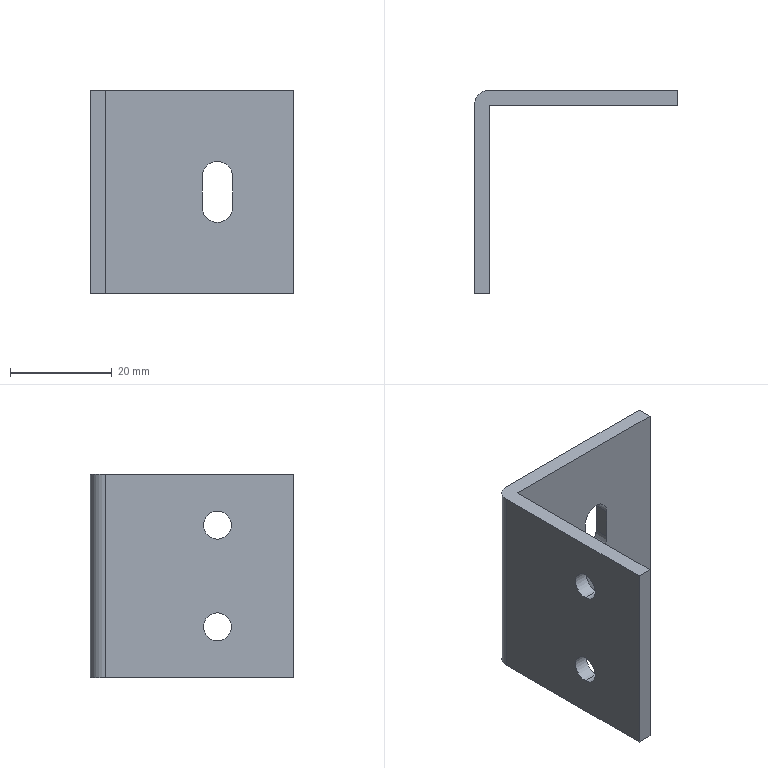Part | STEP file | 0245_212_Blacket | 1 solid | 18 faces | box 40 x 40 x 40 mm | volume 8827 mm3 | plane 10 | cylinder 8 | commonest cylinder face diameters 5.5 x4 6 x4
STEP:
#1=CARTESIAN_POINT('',(0.,0.,0.));
#2=DIRECTION('',(0.,0.,1.));
#3=DIRECTION('',(1.,0.,0.));
#4=AXIS2_PLACEMENT_3D('',#1,#2,#3);
#5=CARTESIAN_POINT('',(3.,15.,12.75));
#6=VERTEX_POINT('',#5);
#7=CARTESIAN_POINT('',(0.,15.,12.75));
#8=VERTEX_POINT('',#7);
#9=CARTESIAN_POINT('',(0.,15.,12.75));
#10=DIRECTION('',(-1.,0.,0.));
#11=VECTOR('',#10,1.);
#12=LINE('',#9,#11);
#13=CARTESIAN_POINT('',(0.,15.,10.));
#14=DIRECTION('',(-1.,0.,0.));
#15=DIRECTION('',(0.,0.,1.));
#16=AXIS2_PLACEMENT_3D('',#13,#14,#15);
#17=CYLINDRICAL_SURFACE('',#16,2.75);
#18=CARTESIAN_POINT('',(6.283,0.));
#19=DIRECTION('',(0.,1.));
#20=VECTOR('',#19,1.);
#21=LINE('',#18,#20);
#22=(GEOMETRIC_REPRESENTATION_CONTEXT(2)PARAMETRIC_REPRESENTATION_CONTEXT()REPRESENTATION_CONTEXT('',''));
#23=DEFINITIONAL_REPRESENTATION('',(#21),#22);
#24=PCURVE('',#17,#23);
#25=CARTESIAN_POINT('',(0.,15.,10.));
#26=DIRECTION('',(-1.,0.,0.));
#27=DIRECTION('',(0.,0.,1.));
#28=AXIS2_PLACEMENT_3D('',#25,#26,#27);
#29=CYLINDRICAL_SURFACE('',#28,2.75);
#30=CARTESIAN_POINT('',(0.,0.));
#31=DIRECTION('',(0.,1.));
#32=VECTOR('',#31,1.);
#33=LINE('',#30,#32);
#34=(GEOMETRIC_REPRESENTATION_CONTEXT(2)PARAMETRIC_REPRESENTATION_CONTEXT()REPRESENTATION_CONTEXT('',''));
#35=DEFINITIONAL_REPRESENTATION('',(#33),#34);
#36=PCURVE('',#29,#35);
#37=SURFACE_CURVE('',#12,(#24,#36),.PCURVE_S1.);
#38=EDGE_CURVE('',#6,#8,#37,.T.);
#39=ORIENTED_EDGE('',*,*,#38,.T.);
#40=CARTESIAN_POINT('',(0.,15.,7.25));
#41=VERTEX_POINT('',#40);
#42=CARTESIAN_POINT('',(0.,15.,10.));
#43=DIRECTION('',(-1.,0.,0.));
#44=DIRECTION('',(0.,0.,1.));
#45=AXIS2_PLACEMENT_3D('',#42,#43,#44);
#46=CIRCLE('',#45,2.75);
#47=CARTESIAN_POINT('',(0.,0.));
#48=DIRECTION('',(1.,0.));
#49=VECTOR('',#48,1.);
#50=LINE('',#47,#49);
#51=(GEOMETRIC_REPRESENTATION_CONTEXT(2)PARAMETRIC_REPRESENTATION_CONTEXT()REPRESENTATION_CONTEXT('',''));
#52=DEFINITIONAL_REPRESENTATION('',(#50),#51);
#53=PCURVE('',#17,#52);
#54=CARTESIAN_POINT('',(0.,0.,20.));
#55=DIRECTION('',(1.,0.,0.));
#56=DIRECTION('',(0.,0.,-1.));
#57=AXIS2_PLACEMENT_3D('',#54,#55,#56);
#58=PLANE('',#57);
#59=CARTESIAN_POINT('',(7.25,15.));
#60=CARTESIAN_POINT('',(7.25,19.763));
#61=CARTESIAN_POINT('',(11.375,17.382));
#62=CARTESIAN_POINT('',(15.5,15.));
#63=CARTESIAN_POINT('',(11.375,12.618));
#64=CARTESIAN_POINT('',(7.25,10.237));
#65=CARTESIAN_POINT('',(7.25,15.));
#66=(BOUNDED_CURVE()B_SPLINE_CURVE(2,(#59,#60,#61,#62,#63,#64,#65),.UNSPECIFIED.,.T.,.F.)B_SPLINE_CURVE_WITH_KNOTS((1,2,2,2,2,1),(-2.094,0.,2.094,4.189,6.283,8.378),.UNSPECIFIED.)CURVE()GEOMETRIC_REPRESENTATION_ITEM()RATIONAL_B_SPLINE_CURVE((1.,0.5,1.,0.5,1.,0.5,1.))REPRESENTATION_ITEM(''));
#67=(GEOMETRIC_REPRESENTATION_CONTEXT(2)PARAMETRIC_REPRESENTATION_CONTEXT()REPRESENTATION_CONTEXT('',''));
#68=DEFINITIONAL_REPRESENTATION('',(#66),#67);
#69=PCURVE('',#58,#68);
#70=SURFACE_CURVE('',#46,(#53,#69),.PCURVE_S1.);
#71=EDGE_CURVE('',#41,#8,#70,.T.);
#72=ORIENTED_EDGE('',*,*,#71,.F.);
#73=CARTESIAN_POINT('',(3.,15.,7.25));
#74=VERTEX_POINT('',#73);
#75=CARTESIAN_POINT('',(0.,15.,7.25));
#76=DIRECTION('',(-1.,0.,0.));
#77=VECTOR('',#76,1.);
#78=LINE('',#75,#77);
#79=CARTESIAN_POINT('',(3.142,0.));
#80=DIRECTION('',(0.,1.));
#81=VECTOR('',#80,1.);
#82=LINE('',#79,#81);
#83=(GEOMETRIC_REPRESENTATION_CONTEXT(2)PARAMETRIC_REPRESENTATION_CONTEXT()REPRESENTATION_CONTEXT('',''));
#84=DEFINITIONAL_REPRESENTATION('',(#82),#83);
#85=PCURVE('',#17,#84);
#86=CARTESIAN_POINT('',(3.142,0.));
#87=DIRECTION('',(0.,1.));
#88=VECTOR('',#87,1.);
#89=LINE('',#86,#88);
#90=(GEOMETRIC_REPRESENTATION_CONTEXT(2)PARAMETRIC_REPRESENTATION_CONTEXT()REPRESENTATION_CONTEXT('',''));
#91=DEFINITIONAL_REPRESENTATION('',(#89),#90);
#92=PCURVE('',#29,#91);
#93=SURFACE_CURVE('',#78,(#85,#92),.PCURVE_S1.);
#94=EDGE_CURVE('',#74,#41,#93,.T.);
#95=ORIENTED_EDGE('',*,*,#94,.F.);
#96=CARTESIAN_POINT('',(3.,15.,10.));
#97=DIRECTION('',(-1.,0.,0.));
#98=DIRECTION('',(0.,-1.,0.));
#99=AXIS2_PLACEMENT_3D('',#96,#97,#98);
#100=CIRCLE('',#99,2.75);
#101=CARTESIAN_POINT('',(-1.571,-3.));
#102=DIRECTION('',(1.,0.));
#103=VECTOR('',#102,1.);
#104=LINE('',#101,#103);
#105=(GEOMETRIC_REPRESENTATION_CONTEXT(2)PARAMETRIC_REPRESENTATION_CONTEXT()REPRESENTATION_CONTEXT('',''));
#106=DEFINITIONAL_REPRESENTATION('',(#104),#105);
#107=PCURVE('',#17,#106);
#108=CARTESIAN_POINT('',(3.,37.,20.));
#109=DIRECTION('',(-1.,0.,0.));
#110=DIRECTION('',(0.,-1.,0.));
#111=AXIS2_PLACEMENT_3D('',#108,#109,#110);
#112=PLANE('',#111);
#113=CARTESIAN_POINT('',(22.,-10.));
#114=DIRECTION('',(1.,0.));
#115=AXIS2_PLACEMENT_2D('',#113,#114);
#116=CIRCLE('',#115,2.75);
#117=(GEOMETRIC_REPRESENTATION_CONTEXT(2)PARAMETRIC_REPRESENTATION_CONTEXT()REPRESENTATION_CONTEXT('',''));
#118=DEFINITIONAL_REPRESENTATION('',(#116),#117);
#119=PCURVE('',#112,#118);
#120=SURFACE_CURVE('',#100,(#107,#119),.PCURVE_S1.);
#121=EDGE_CURVE('',#74,#6,#120,.T.);
#122=ORIENTED_EDGE('',*,*,#121,.T.);
#123=EDGE_LOOP('',(#39,#72,#95,#122));
#124=FACE_BOUND('',#123,.F.);
#125=ADVANCED_FACE('',(#124),#17,.F.);
#126=CARTESIAN_POINT('',(3.,15.,-7.25));
#127=VERTEX_POINT('',#126);
#128=CARTESIAN_POINT('',(0.,15.,-7.25));
#129=VERTEX_POINT('',#128);
#130=CARTESIAN_POINT('',(0.,15.,-7.25));
#131=DIRECTION('',(-1.,0.,0.));
#132=VECTOR('',#131,1.);
#133=LINE('',#130,#132);
#134=CARTESIAN_POINT('',(0.,15.,-10.));
#135=DIRECTION('',(-1.,0.,0.));
#136=DIRECTION('',(0.,0.,1.));
#137=AXIS2_PLACEMENT_3D('',#134,#135,#136);
#138=CYLINDRICAL_SURFACE('',#137,2.75);
#139=CARTESIAN_POINT('',(6.283,0.));
#140=DIRECTION('',(0.,1.));
#141=VECTOR('',#140,1.);
#142=LINE('',#139,#141);
#143=(GEOMETRIC_REPRESENTATION_CONTEXT(2)PARAMETRIC_REPRESENTATION_CONTEXT()REPRESENTATION_CONTEXT('',''));
#144=DEFINITIONAL_REPRESENTATION('',(#142),#143);
#145=PCURVE('',#138,#144);
#146=CARTESIAN_POINT('',(0.,15.,-10.));
#147=DIRECTION('',(-1.,0.,0.));
#148=DIRECTION('',(0.,0.,1.));
#149=AXIS2_PLACEMENT_3D('',#146,#147,#148);
#150=CYLINDRICAL_SURFACE('',#149,2.75);
#151=CARTESIAN_POINT('',(0.,0.));
#152=DIRECTION('',(0.,1.));
#153=VECTOR('',#152,1.);
#154=LINE('',#151,#153);
#155=(GEOMETRIC_REPRESENTATION_CONTEXT(2)PARAMETRIC_REPRESENTATION_CONTEXT()REPRESENTATION_CONTEXT('',''));
#156=DEFINITIONAL_REPRESENTATION('',(#154),#155);
#157=PCURVE('',#150,#156);
#158=SURFACE_CURVE('',#133,(#145,#157),.PCURVE_S1.);
#159=EDGE_CURVE('',#127,#129,#158,.T.);
#160=ORIENTED_EDGE('',*,*,#159,.T.);
#161=CARTESIAN_POINT('',(0.,15.,-12.75));
#162=VERTEX_POINT('',#161);
#163=CARTESIAN_POINT('',(0.,15.,-10.));
#164=DIRECTION('',(-1.,0.,0.));
#165=DIRECTION('',(0.,0.,1.));
#166=AXIS2_PLACEMENT_3D('',#163,#164,#165);
#167=CIRCLE('',#166,2.75);
#168=CARTESIAN_POINT('',(0.,0.));
#169=DIRECTION('',(1.,0.));
#170=VECTOR('',#169,1.);
#171=LINE('',#168,#170);
#172=(GEOMETRIC_REPRESENTATION_CONTEXT(2)PARAMETRIC_REPRESENTATION_CONTEXT()REPRESENTATION_CONTEXT('',''));
#173=DEFINITIONAL_REPRESENTATION('',(#171),#172);
#174=PCURVE('',#138,#173);
#175=CARTESIAN_POINT('',(27.25,15.));
#176=CARTESIAN_POINT('',(27.25,19.763));
#177=CARTESIAN_POINT('',(31.375,17.382));
#178=CARTESIAN_POINT('',(35.5,15.));
#179=CARTESIAN_POINT('',(31.375,12.618));
#180=CARTESIAN_POINT('',(27.25,10.237));
#181=CARTESIAN_POINT('',(27.25,15.));
#182=(BOUNDED_CURVE()B_SPLINE_CURVE(2,(#175,#176,#177,#178,#179,#180,#181),.UNSPECIFIED.,.T.,.F.)B_SPLINE_CURVE_WITH_KNOTS((1,2,2,2,2,1),(-2.094,0.,2.094,4.189,6.283,8.378),.UNSPECIFIED.)CURVE()GEOMETRIC_REPRESENTATION_ITEM()RATIONAL_B_SPLINE_CURVE((1.,0.5,1.,0.5,1.,0.5,1.))REPRESENTATION_ITEM(''));
#183=(GEOMETRIC_REPRESENTATION_CONTEXT(2)PARAMETRIC_REPRESENTATION_CONTEXT()REPRESENTATION_CONTEXT('',''));
#184=DEFINITIONAL_REPRESENTATION('',(#182),#183);
#185=PCURVE('',#58,#184);
#186=SURFACE_CURVE('',#167,(#174,#185),.PCURVE_S1.);
#187=EDGE_CURVE('',#162,#129,#186,.T.);
#188=ORIENTED_EDGE('',*,*,#187,.F.);
#189=CARTESIAN_POINT('',(3.,15.,-12.75));
#190=VERTEX_POINT('',#189);
#191=CARTESIAN_POINT('',(0.,15.,-12.75));
#192=DIRECTION('',(-1.,0.,0.));
#193=VECTOR('',#192,1.);
#194=LINE('',#191,#193);
#195=CARTESIAN_POINT('',(3.142,0.));
#196=DIRECTION('',(0.,1.));
#197=VECTOR('',#196,1.);
#198=LINE('',#195,#197);
#199=(GEOMETRIC_REPRESENTATION_CONTEXT(2)PARAMETRIC_REPRESENTATION_CONTEXT()REPRESENTATION_CONTEXT('',''));
#200=DEFINITIONAL_REPRESENTATION('',(#198),#199);
#201=PCURVE('',#138,#200);
#202=CARTESIAN_POINT('',(3.142,0.));
#203=DIRECTION('',(0.,1.));
#204=VECTOR('',#203,1.);
#205=LINE('',#202,#204);
#206=(GEOMETRIC_REPRESENTATION_CONTEXT(2)PARAMETRIC_REPRESENTATION_CONTEXT()REPRESENTATION_CONTEXT('',''));
#207=DEFINITIONAL_REPRESENTATION('',(#205),#206);
#208=PCURVE('',#150,#207);
#209=SURFACE_CURVE('',#194,(#201,#208),.PCURVE_S1.);
#210=EDGE_CURVE('',#190,#162,#209,.T.);
#211=ORIENTED_EDGE('',*,*,#210,.F.);
#212=CARTESIAN_POINT('',(3.,15.,-10.));
#213=DIRECTION('',(-1.,0.,0.));
#214=DIRECTION('',(0.,-1.,0.));
#215=AXIS2_PLACEMENT_3D('',#212,#213,#214);
#216=CIRCLE('',#215,2.75);
#217=CARTESIAN_POINT('',(-1.571,-3.));
#218=DIRECTION('',(1.,0.));
#219=VECTOR('',#218,1.);
#220=LINE('',#217,#219);
#221=(GEOMETRIC_REPRESENTATION_CONTEXT(2)PARAMETRIC_REPRESENTATION_CONTEXT()REPRESENTATION_CONTEXT('',''));
#222=DEFINITIONAL_REPRESENTATION('',(#220),#221);
#223=PCURVE('',#138,#222);
#224=CARTESIAN_POINT('',(22.,-30.));
#225=DIRECTION('',(1.,0.));
#226=AXIS2_PLACEMENT_2D('',#224,#225);
#227=CIRCLE('',#226,2.75);
#228=(GEOMETRIC_REPRESENTATION_CONTEXT(2)PARAMETRIC_REPRESENTATION_CONTEXT()REPRESENTATION_CONTEXT('',''));
#229=DEFINITIONAL_REPRESENTATION('',(#227),#228);
#230=PCURVE('',#112,#229);
#231=SURFACE_CURVE('',#216,(#223,#230),.PCURVE_S1.);
#232=EDGE_CURVE('',#190,#127,#231,.T.);
#233=ORIENTED_EDGE('',*,*,#232,.T.);
#234=EDGE_LOOP('',(#160,#188,#211,#233));
#235=FACE_BOUND('',#234,.F.);
#236=ADVANCED_FACE('',(#235),#138,.F.);
#237=CARTESIAN_POINT('',(28.,37.,3.));
#238=VERTEX_POINT('',#237);
#239=CARTESIAN_POINT('',(28.,40.,3.));
#240=VERTEX_POINT('',#239);
#241=CARTESIAN_POINT('',(28.,0.,3.));
#242=DIRECTION('',(0.,1.,0.));
#243=VECTOR('',#242,1.);
#244=LINE('',#241,#243);
#245=CARTESIAN_POINT('',(25.,0.,3.));
#246=DIRECTION('',(0.,1.,0.));
#247=DIRECTION('',(0.,0.,1.));
#248=AXIS2_PLACEMENT_3D('',#245,#246,#247);
#249=CYLINDRICAL_SURFACE('',#248,3.);
#250=CARTESIAN_POINT('',(1.571,0.));
#251=DIRECTION('',(0.,1.));
#252=VECTOR('',#251,1.);
#253=LINE('',#250,#252);
#254=(GEOMETRIC_REPRESENTATION_CONTEXT(2)PARAMETRIC_REPRESENTATION_CONTEXT()REPRESENTATION_CONTEXT('',''));
#255=DEFINITIONAL_REPRESENTATION('',(#253),#254);
#256=PCURVE('',#249,#255);
#257=CARTESIAN_POINT('',(28.,0.,-3.));
#258=DIRECTION('',(1.,0.,0.));
#259=DIRECTION('',(0.,0.,-1.));
#260=AXIS2_PLACEMENT_3D('',#257,#258,#259);
#261=PLANE('',#260);
#262=CARTESIAN_POINT('',(-6.,0.));
#263=DIRECTION('',(0.,1.));
#264=VECTOR('',#263,1.);
#265=LINE('',#262,#264);
#266=(GEOMETRIC_REPRESENTATION_CONTEXT(2)PARAMETRIC_REPRESENTATION_CONTEXT()REPRESENTATION_CONTEXT('',''));
#267=DEFINITIONAL_REPRESENTATION('',(#265),#266);
#268=PCURVE('',#261,#267);
#269=SURFACE_CURVE('',#244,(#256,#268),.PCURVE_S1.);
#270=EDGE_CURVE('',#238,#240,#269,.T.);
#271=ORIENTED_EDGE('',*,*,#270,.T.);
#272=CARTESIAN_POINT('',(25.,40.,6.));
#273=VERTEX_POINT('',#272);
#274=CARTESIAN_POINT('',(25.,40.,3.));
#275=DIRECTION('',(0.,1.,0.));
#276=DIRECTION('',(0.,0.,1.));
#277=AXIS2_PLACEMENT_3D('',#274,#275,#276);
#278=CIRCLE('',#277,3.);
#279=CARTESIAN_POINT('',(0.,40.));
#280=DIRECTION('',(1.,0.));
#281=VECTOR('',#280,1.);
#282=LINE('',#279,#281);
#283=(GEOMETRIC_REPRESENTATION_CONTEXT(2)PARAMETRIC_REPRESENTATION_CONTEXT()REPRESENTATION_CONTEXT('',''));
#284=DEFINITIONAL_REPRESENTATION('',(#282),#283);
#285=PCURVE('',#249,#284);
#286=CARTESIAN_POINT('',(0.,40.,20.));
#287=DIRECTION('',(0.,-1.,0.));
#288=DIRECTION('',(0.,0.,-1.));
#289=AXIS2_PLACEMENT_3D('',#286,#287,#288);
#290=PLANE('',#289);
#291=CARTESIAN_POINT('',(14.,25.));
#292=CARTESIAN_POINT('',(14.,30.196));
#293=CARTESIAN_POINT('',(18.5,27.598));
#294=CARTESIAN_POINT('',(23.,25.));
#295=CARTESIAN_POINT('',(18.5,22.402));
#296=CARTESIAN_POINT('',(14.,19.804));
#297=CARTESIAN_POINT('',(14.,25.));
#298=(BOUNDED_CURVE()B_SPLINE_CURVE(2,(#291,#292,#293,#294,#295,#296,#297),.UNSPECIFIED.,.T.,.F.)B_SPLINE_CURVE_WITH_KNOTS((1,2,2,2,2,1),(-2.094,0.,2.094,4.189,6.283,8.378),.UNSPECIFIED.)CURVE()GEOMETRIC_REPRESENTATION_ITEM()RATIONAL_B_SPLINE_CURVE((1.,0.5,1.,0.5,1.,0.5,1.))REPRESENTATION_ITEM(''));
#299=(GEOMETRIC_REPRESENTATION_CONTEXT(2)PARAMETRIC_REPRESENTATION_CONTEXT()REPRESENTATION_CONTEXT('',''));
#300=DEFINITIONAL_REPRESENTATION('',(#298),#299);
#301=PCURVE('',#290,#300);
#302=SURFACE_CURVE('',#278,(#285,#301),.PCURVE_S1.);
#303=EDGE_CURVE('',#273,#240,#302,.T.);
#304=ORIENTED_EDGE('',*,*,#303,.F.);
#305=CARTESIAN_POINT('',(25.,37.,6.));
#306=VERTEX_POINT('',#305);
#307=CARTESIAN_POINT('',(25.,0.,6.));
#308=DIRECTION('',(0.,1.,0.));
#309=VECTOR('',#308,1.);
#310=LINE('',#307,#309);
#311=CARTESIAN_POINT('',(0.,0.));
#312=DIRECTION('',(0.,1.));
#313=VECTOR('',#312,1.);
#314=LINE('',#311,#313);
#315=(GEOMETRIC_REPRESENTATION_CONTEXT(2)PARAMETRIC_REPRESENTATION_CONTEXT()REPRESENTATION_CONTEXT('',''));
#316=DEFINITIONAL_REPRESENTATION('',(#314),#315);
#317=PCURVE('',#249,#316);
#318=CARTESIAN_POINT('',(25.,0.,3.));
#319=DIRECTION('',(0.,1.,0.));
#320=DIRECTION('',(0.,0.,1.));
#321=AXIS2_PLACEMENT_3D('',#318,#319,#320);
#322=CYLINDRICAL_SURFACE('',#321,3.);
#323=CARTESIAN_POINT('',(6.283,0.));
#324=DIRECTION('',(0.,1.));
#325=VECTOR('',#324,1.);
#326=LINE('',#323,#325);
#327=(GEOMETRIC_REPRESENTATION_CONTEXT(2)PARAMETRIC_REPRESENTATION_CONTEXT()REPRESENTATION_CONTEXT('',''));
#328=DEFINITIONAL_REPRESENTATION('',(#326),#327);
#329=PCURVE('',#322,#328);
#330=SURFACE_CURVE('',#310,(#317,#329),.PCURVE_S1.);
#331=EDGE_CURVE('',#306,#273,#330,.T.);
#332=ORIENTED_EDGE('',*,*,#331,.F.);
#333=CARTESIAN_POINT('',(25.,37.,3.));
#334=DIRECTION('',(0.,1.,0.));
#335=DIRECTION('',(-1.,0.,0.));
#336=AXIS2_PLACEMENT_3D('',#333,#334,#335);
#337=CIRCLE('',#336,3.);
#338=CARTESIAN_POINT('',(-1.571,37.));
#339=DIRECTION('',(1.,0.));
#340=VECTOR('',#339,1.);
#341=LINE('',#338,#340);
#342=(GEOMETRIC_REPRESENTATION_CONTEXT(2)PARAMETRIC_REPRESENTATION_CONTEXT()REPRESENTATION_CONTEXT('',''));
#343=DEFINITIONAL_REPRESENTATION('',(#341),#342);
#344=PCURVE('',#249,#343);
#345=CARTESIAN_POINT('',(40.,37.,20.));
#346=DIRECTION('',(0.,1.,0.));
#347=DIRECTION('',(-1.,0.,0.));
#348=AXIS2_PLACEMENT_3D('',#345,#346,#347);
#349=PLANE('',#348);
#350=CARTESIAN_POINT('',(15.,-17.));
#351=DIRECTION('',(1.,0.));
#352=AXIS2_PLACEMENT_2D('',#350,#351);
#353=CIRCLE('',#352,3.);
#354=(GEOMETRIC_REPRESENTATION_CONTEXT(2)PARAMETRIC_REPRESENTATION_CONTEXT()REPRESENTATION_CONTEXT('',''));
#355=DEFINITIONAL_REPRESENTATION('',(#353),#354);
#356=PCURVE('',#349,#355);
#357=SURFACE_CURVE('',#337,(#344,#356),.PCURVE_S1.);
#358=EDGE_CURVE('',#306,#238,#357,.T.);
#359=ORIENTED_EDGE('',*,*,#358,.T.);
#360=EDGE_LOOP('',(#271,#304,#332,#359));
#361=FACE_BOUND('',#360,.F.);
#362=ADVANCED_FACE('',(#361),#249,.F.);
#363=CARTESIAN_POINT('',(0.,0.,-20.));
#364=VERTEX_POINT('',#363);
#365=CARTESIAN_POINT('',(3.,0.,-20.));
#366=VERTEX_POINT('',#365);
#367=CARTESIAN_POINT('',(3.,0.,-20.));
#368=DIRECTION('',(1.,0.,0.));
#369=VECTOR('',#368,1.);
#370=LINE('',#367,#369);
#371=CARTESIAN_POINT('',(3.,0.,20.));
#372=DIRECTION('',(0.,1.,0.));
#373=DIRECTION('',(-1.,0.,0.));
#374=AXIS2_PLACEMENT_3D('',#371,#372,#373);
#375=PLANE('',#374);
#376=CARTESIAN_POINT('',(0.,-40.));
#377=DIRECTION('',(-1.,0.));
#378=VECTOR('',#377,1.);
#379=LINE('',#376,#378);
#380=(GEOMETRIC_REPRESENTATION_CONTEXT(2)PARAMETRIC_REPRESENTATION_CONTEXT()REPRESENTATION_CONTEXT('',''));
#381=DEFINITIONAL_REPRESENTATION('',(#379),#380);
#382=PCURVE('',#375,#381);
#383=CARTESIAN_POINT('',(0.,0.,-20.));
#384=DIRECTION('',(0.,0.,-1.));
#385=DIRECTION('',(-1.,0.,0.));
#386=AXIS2_PLACEMENT_3D('',#383,#384,#385);
#387=PLANE('',#386);
#388=CARTESIAN_POINT('',(-3.,0.));
#389=DIRECTION('',(-1.,0.));
#390=VECTOR('',#389,1.);
#391=LINE('',#388,#390);
#392=(GEOMETRIC_REPRESENTATION_CONTEXT(2)PARAMETRIC_REPRESENTATION_CONTEXT()REPRESENTATION_CONTEXT('',''));
#393=DEFINITIONAL_REPRESENTATION('',(#391),#392);
#394=PCURVE('',#387,#393);
#395=SURFACE_CURVE('',#370,(#382,#394),.PCURVE_S1.);
#396=EDGE_CURVE('',#364,#366,#395,.T.);
#397=ORIENTED_EDGE('',*,*,#396,.T.);
#398=CARTESIAN_POINT('',(3.,0.,20.));
#399=VERTEX_POINT('',#398);
#400=CARTESIAN_POINT('',(3.,0.,20.));
#401=DIRECTION('',(0.,0.,-1.));
#402=VECTOR('',#401,1.);
#403=LINE('',#400,#402);
#404=CARTESIAN_POINT('',(0.,0.));
#405=DIRECTION('',(0.,-1.));
#406=VECTOR('',#405,1.);
#407=LINE('',#404,#406);
#408=(GEOMETRIC_REPRESENTATION_CONTEXT(2)PARAMETRIC_REPRESENTATION_CONTEXT()REPRESENTATION_CONTEXT('',''));
#409=DEFINITIONAL_REPRESENTATION('',(#407),#408);
#410=PCURVE('',#375,#409);
#411=CARTESIAN_POINT('',(37.,0.));
#412=DIRECTION('',(0.,-1.));
#413=VECTOR('',#412,1.);
#414=LINE('',#411,#413);
#415=(GEOMETRIC_REPRESENTATION_CONTEXT(2)PARAMETRIC_REPRESENTATION_CONTEXT()REPRESENTATION_CONTEXT('',''));
#416=DEFINITIONAL_REPRESENTATION('',(#414),#415);
#417=PCURVE('',#112,#416);
#418=SURFACE_CURVE('',#403,(#410,#417),.PCURVE_S1.);
#419=EDGE_CURVE('',#399,#366,#418,.T.);
#420=ORIENTED_EDGE('',*,*,#419,.F.);
#421=CARTESIAN_POINT('',(0.,0.,20.));
#422=VERTEX_POINT('',#421);
#423=CARTESIAN_POINT('',(3.,0.,20.));
#424=DIRECTION('',(1.,0.,0.));
#425=VECTOR('',#424,1.);
#426=LINE('',#423,#425);
#427=CARTESIAN_POINT('',(0.,0.));
#428=DIRECTION('',(-1.,0.));
#429=VECTOR('',#428,1.);
#430=LINE('',#427,#429);
#431=(GEOMETRIC_REPRESENTATION_CONTEXT(2)PARAMETRIC_REPRESENTATION_CONTEXT()REPRESENTATION_CONTEXT('',''));
#432=DEFINITIONAL_REPRESENTATION('',(#430),#431);
#433=PCURVE('',#375,#432);
#434=CARTESIAN_POINT('',(0.,0.,20.));
#435=DIRECTION('',(0.,0.,-1.));
#436=DIRECTION('',(-1.,0.,0.));
#437=AXIS2_PLACEMENT_3D('',#434,#435,#436);
#438=PLANE('',#437);
#439=CARTESIAN_POINT('',(-3.,0.));
#440=DIRECTION('',(-1.,0.));
#441=VECTOR('',#440,1.);
#442=LINE('',#439,#441);
#443=(GEOMETRIC_REPRESENTATION_CONTEXT(2)PARAMETRIC_REPRESENTATION_CONTEXT()REPRESENTATION_CONTEXT('',''));
#444=DEFINITIONAL_REPRESENTATION('',(#442),#443);
#445=PCURVE('',#438,#444);
#446=SURFACE_CURVE('',#426,(#433,#445),.PCURVE_S1.);
#447=EDGE_CURVE('',#422,#399,#446,.T.);
#448=ORIENTED_EDGE('',*,*,#447,.F.);
#449=CARTESIAN_POINT('',(0.,0.,20.));
#450=DIRECTION('',(0.,0.,-1.));
#451=VECTOR('',#450,1.);
#452=LINE('',#449,#451);
#453=CARTESIAN_POINT('',(3.,0.));
#454=DIRECTION('',(0.,-1.));
#455=VECTOR('',#454,1.);
#456=LINE('',#453,#455);
#457=(GEOMETRIC_REPRESENTATION_CONTEXT(2)PARAMETRIC_REPRESENTATION_CONTEXT()REPRESENTATION_CONTEXT('',''));
#458=DEFINITIONAL_REPRESENTATION('',(#456),#457);
#459=PCURVE('',#375,#458);
#460=CARTESIAN_POINT('',(0.,0.));
#461=DIRECTION('',(1.,0.));
#462=VECTOR('',#461,1.);
#463=LINE('',#460,#462);
#464=(GEOMETRIC_REPRESENTATION_CONTEXT(2)PARAMETRIC_REPRESENTATION_CONTEXT()REPRESENTATION_CONTEXT('',''));
#465=DEFINITIONAL_REPRESENTATION('',(#463),#464);
#466=PCURVE('',#58,#465);
#467=SURFACE_CURVE('',#452,(#459,#466),.PCURVE_S1.);
#468=EDGE_CURVE('',#422,#364,#467,.T.);
#469=ORIENTED_EDGE('',*,*,#468,.T.);
#470=EDGE_LOOP('',(#397,#420,#448,#469));
#471=FACE_BOUND('',#470,.T.);
#472=ADVANCED_FACE('',(#471),#375,.F.);
#473=CARTESIAN_POINT('',(3.,15.,10.));
#474=DIRECTION('',(-1.,0.,0.));
#475=DIRECTION('',(0.,-1.,0.));
#476=AXIS2_PLACEMENT_3D('',#473,#474,#475);
#477=CIRCLE('',#476,2.75);
#478=CARTESIAN_POINT('',(22.,-10.));
#479=DIRECTION('',(1.,0.));
#480=AXIS2_PLACEMENT_2D('',#478,#479);
#481=CIRCLE('',#480,2.75);
#482=(GEOMETRIC_REPRESENTATION_CONTEXT(2)PARAMETRIC_REPRESENTATION_CONTEXT()REPRESENTATION_CONTEXT('',''));
#483=DEFINITIONAL_REPRESENTATION('',(#481),#482);
#484=PCURVE('',#112,#483);
#485=CARTESIAN_POINT('',(-1.571,-3.));
#486=DIRECTION('',(1.,0.));
#487=VECTOR('',#486,1.);
#488=LINE('',#485,#487);
#489=(GEOMETRIC_REPRESENTATION_CONTEXT(2)PARAMETRIC_REPRESENTATION_CONTEXT()REPRESENTATION_CONTEXT('',''));
#490=DEFINITIONAL_REPRESENTATION('',(#488),#489);
#491=PCURVE('',#29,#490);
#492=SURFACE_CURVE('',#477,(#484,#491),.PCURVE_S1.);
#493=EDGE_CURVE('',#6,#74,#492,.T.);
#494=ORIENTED_EDGE('',*,*,#493,.T.);
#495=ORIENTED_EDGE('',*,*,#121,.T.);
#496=EDGE_LOOP('',(#494,#495));
#497=FACE_BOUND('',#496,.T.);
#498=CARTESIAN_POINT('',(3.,15.,-10.));
#499=DIRECTION('',(-1.,0.,0.));
#500=DIRECTION('',(0.,-1.,0.));
#501=AXIS2_PLACEMENT_3D('',#498,#499,#500);
#502=CIRCLE('',#501,2.75);
#503=CARTESIAN_POINT('',(22.,-30.));
#504=DIRECTION('',(1.,0.));
#505=AXIS2_PLACEMENT_2D('',#503,#504);
#506=CIRCLE('',#505,2.75);
#507=(GEOMETRIC_REPRESENTATION_CONTEXT(2)PARAMETRIC_REPRESENTATION_CONTEXT()REPRESENTATION_CONTEXT('',''));
#508=DEFINITIONAL_REPRESENTATION('',(#506),#507);
#509=PCURVE('',#112,#508);
#510=CARTESIAN_POINT('',(-1.571,-3.));
#511=DIRECTION('',(1.,0.));
#512=VECTOR('',#511,1.);
#513=LINE('',#510,#512);
#514=(GEOMETRIC_REPRESENTATION_CONTEXT(2)PARAMETRIC_REPRESENTATION_CONTEXT()REPRESENTATION_CONTEXT('',''));
#515=DEFINITIONAL_REPRESENTATION('',(#513),#514);
#516=PCURVE('',#150,#515);
#517=SURFACE_CURVE('',#502,(#509,#516),.PCURVE_S1.);
#518=EDGE_CURVE('',#127,#190,#517,.T.);
#519=ORIENTED_EDGE('',*,*,#518,.T.);
#520=ORIENTED_EDGE('',*,*,#232,.T.);
#521=EDGE_LOOP('',(#519,#520));
#522=FACE_BOUND('',#521,.T.);
#523=CARTESIAN_POINT('',(3.,37.,-20.));
#524=VERTEX_POINT('',#523);
#525=CARTESIAN_POINT('',(3.,37.,-20.));
#526=DIRECTION('',(0.,1.,0.));
#527=VECTOR('',#526,1.);
#528=LINE('',#525,#527);
#529=CARTESIAN_POINT('',(0.,-40.));
#530=DIRECTION('',(-1.,0.));
#531=VECTOR('',#530,1.);
#532=LINE('',#529,#531);
#533=(GEOMETRIC_REPRESENTATION_CONTEXT(2)PARAMETRIC_REPRESENTATION_CONTEXT()REPRESENTATION_CONTEXT('',''));
#534=DEFINITIONAL_REPRESENTATION('',(#532),#533);
#535=PCURVE('',#112,#534);
#536=CARTESIAN_POINT('',(-3.,37.));
#537=DIRECTION('',(0.,1.));
#538=VECTOR('',#537,1.);
#539=LINE('',#536,#538);
#540=(GEOMETRIC_REPRESENTATION_CONTEXT(2)PARAMETRIC_REPRESENTATION_CONTEXT()REPRESENTATION_CONTEXT('',''));
#541=DEFINITIONAL_REPRESENTATION('',(#539),#540);
#542=PCURVE('',#387,#541);
#543=SURFACE_CURVE('',#528,(#535,#542),.PCURVE_S1.);
#544=EDGE_CURVE('',#366,#524,#543,.T.);
#545=ORIENTED_EDGE('',*,*,#544,.T.);
#546=CARTESIAN_POINT('',(3.,37.,20.));
#547=VERTEX_POINT('',#546);
#548=CARTESIAN_POINT('',(3.,37.,20.));
#549=DIRECTION('',(0.,0.,-1.));
#550=VECTOR('',#549,1.);
#551=LINE('',#548,#550);
#552=CARTESIAN_POINT('',(0.,0.));
#553=DIRECTION('',(0.,-1.));
#554=VECTOR('',#553,1.);
#555=LINE('',#552,#554);
#556=(GEOMETRIC_REPRESENTATION_CONTEXT(2)PARAMETRIC_REPRESENTATION_CONTEXT()REPRESENTATION_CONTEXT('',''));
#557=DEFINITIONAL_REPRESENTATION('',(#555),#556);
#558=PCURVE('',#112,#557);
#559=CARTESIAN_POINT('',(37.,0.));
#560=DIRECTION('',(0.,-1.));
#561=VECTOR('',#560,1.);
#562=LINE('',#559,#561);
#563=(GEOMETRIC_REPRESENTATION_CONTEXT(2)PARAMETRIC_REPRESENTATION_CONTEXT()REPRESENTATION_CONTEXT('',''));
#564=DEFINITIONAL_REPRESENTATION('',(#562),#563);
#565=PCURVE('',#349,#564);
#566=SURFACE_CURVE('',#551,(#558,#565),.PCURVE_S1.);
#567=EDGE_CURVE('',#547,#524,#566,.T.);
#568=ORIENTED_EDGE('',*,*,#567,.F.);
#569=CARTESIAN_POINT('',(3.,37.,20.));
#570=DIRECTION('',(0.,1.,0.));
#571=VECTOR('',#570,1.);
#572=LINE('',#569,#571);
#573=CARTESIAN_POINT('',(0.,0.));
#574=DIRECTION('',(-1.,0.));
#575=VECTOR('',#574,1.);
#576=LINE('',#573,#575);
#577=(GEOMETRIC_REPRESENTATION_CONTEXT(2)PARAMETRIC_REPRESENTATION_CONTEXT()REPRESENTATION_CONTEXT('',''));
#578=DEFINITIONAL_REPRESENTATION('',(#576),#577);
#579=PCURVE('',#112,#578);
#580=CARTESIAN_POINT('',(-3.,37.));
#581=DIRECTION('',(0.,1.));
#582=VECTOR('',#581,1.);
#583=LINE('',#580,#582);
#584=(GEOMETRIC_REPRESENTATION_CONTEXT(2)PARAMETRIC_REPRESENTATION_CONTEXT()REPRESENTATION_CONTEXT('',''));
#585=DEFINITIONAL_REPRESENTATION('',(#583),#584);
#586=PCURVE('',#438,#585);
#587=SURFACE_CURVE('',#572,(#579,#586),.PCURVE_S1.);
#588=EDGE_CURVE('',#399,#547,#587,.T.);
#589=ORIENTED_EDGE('',*,*,#588,.F.);
#590=ORIENTED_EDGE('',*,*,#419,.T.);
#591=EDGE_LOOP('',(#545,#568,#589,#590));
#592=FACE_BOUND('',#591,.T.);
#593=ADVANCED_FACE('',(#497,#522,#592),#112,.F.);
#594=CARTESIAN_POINT('',(28.,37.,-3.));
#595=VERTEX_POINT('',#594);
#596=CARTESIAN_POINT('',(28.,37.,20.));
#597=DIRECTION('',(0.,0.,-1.));
#598=VECTOR('',#597,1.);
#599=LINE('',#596,#598);
#600=CARTESIAN_POINT('',(12.,0.));
#601=DIRECTION('',(0.,-1.));
#602=VECTOR('',#601,1.);
#603=LINE('',#600,#602);
#604=(GEOMETRIC_REPRESENTATION_CONTEXT(2)PARAMETRIC_REPRESENTATION_CONTEXT()REPRESENTATION_CONTEXT('',''));
#605=DEFINITIONAL_REPRESENTATION('',(#603),#604);
#606=PCURVE('',#349,#605);
#607=CARTESIAN_POINT('',(-23.,37.));
#608=DIRECTION('',(1.,0.));
#609=VECTOR('',#608,1.);
#610=LINE('',#607,#609);
#611=(GEOMETRIC_REPRESENTATION_CONTEXT(2)PARAMETRIC_REPRESENTATION_CONTEXT()REPRESENTATION_CONTEXT('',''));
#612=DEFINITIONAL_REPRESENTATION('',(#610),#611);
#613=PCURVE('',#261,#612);
#614=SURFACE_CURVE('',#599,(#606,#613),.PCURVE_S1.);
#615=EDGE_CURVE('',#238,#595,#614,.T.);
#616=ORIENTED_EDGE('',*,*,#615,.T.);
#617=CARTESIAN_POINT('',(22.,37.,-3.));
#618=VERTEX_POINT('',#617);
#619=CARTESIAN_POINT('',(25.,37.,-3.));
#620=DIRECTION('',(0.,1.,0.));
#621=DIRECTION('',(-1.,0.,0.));
#622=AXIS2_PLACEMENT_3D('',#619,#620,#621);
#623=CIRCLE('',#622,3.);
#624=CARTESIAN_POINT('',(15.,-23.));
#625=DIRECTION('',(1.,0.));
#626=AXIS2_PLACEMENT_2D('',#624,#625);
#627=CIRCLE('',#626,3.);
#628=(GEOMETRIC_REPRESENTATION_CONTEXT(2)PARAMETRIC_REPRESENTATION_CONTEXT()REPRESENTATION_CONTEXT('',''));
#629=DEFINITIONAL_REPRESENTATION('',(#627),#628);
#630=PCURVE('',#349,#629);
#631=CARTESIAN_POINT('',(25.,0.,-3.));
#632=DIRECTION('',(0.,1.,0.));
#633=DIRECTION('',(0.,0.,1.));
#634=AXIS2_PLACEMENT_3D('',#631,#632,#633);
#635=CYLINDRICAL_SURFACE('',#634,3.);
#636=CARTESIAN_POINT('',(-1.571,37.));
#637=DIRECTION('',(1.,0.));
#638=VECTOR('',#637,1.);
#639=LINE('',#636,#638);
#640=(GEOMETRIC_REPRESENTATION_CONTEXT(2)PARAMETRIC_REPRESENTATION_CONTEXT()REPRESENTATION_CONTEXT('',''));
#641=DEFINITIONAL_REPRESENTATION('',(#639),#640);
#642=PCURVE('',#635,#641);
#643=SURFACE_CURVE('',#623,(#630,#642),.PCURVE_S1.);
#644=EDGE_CURVE('',#595,#618,#643,.T.);
#645=ORIENTED_EDGE('',*,*,#644,.T.);
#646=CARTESIAN_POINT('',(22.,37.,3.));
#647=VERTEX_POINT('',#646);
#648=CARTESIAN_POINT('',(22.,37.,20.));
#649=DIRECTION('',(0.,0.,1.));
#650=VECTOR('',#649,1.);
#651=LINE('',#648,#650);
#652=CARTESIAN_POINT('',(18.,0.));
#653=DIRECTION('',(0.,1.));
#654=VECTOR('',#653,1.);
#655=LINE('',#652,#654);
#656=(GEOMETRIC_REPRESENTATION_CONTEXT(2)PARAMETRIC_REPRESENTATION_CONTEXT()REPRESENTATION_CONTEXT('',''));
#657=DEFINITIONAL_REPRESENTATION('',(#655),#656);
#658=PCURVE('',#349,#657);
#659=CARTESIAN_POINT('',(22.,0.,-3.));
#660=DIRECTION('',(-1.,0.,0.));
#661=DIRECTION('',(0.,0.,1.));
#662=AXIS2_PLACEMENT_3D('',#659,#660,#661);
#663=PLANE('',#662);
#664=CARTESIAN_POINT('',(23.,37.));
#665=DIRECTION('',(1.,0.));
#666=VECTOR('',#665,1.);
#667=LINE('',#664,#666);
#668=(GEOMETRIC_REPRESENTATION_CONTEXT(2)PARAMETRIC_REPRESENTATION_CONTEXT()REPRESENTATION_CONTEXT('',''));
#669=DEFINITIONAL_REPRESENTATION('',(#667),#668);
#670=PCURVE('',#663,#669);
#671=SURFACE_CURVE('',#651,(#658,#670),.PCURVE_S1.);
#672=EDGE_CURVE('',#618,#647,#671,.T.);
#673=ORIENTED_EDGE('',*,*,#672,.T.);
#674=CARTESIAN_POINT('',(25.,37.,3.));
#675=DIRECTION('',(0.,1.,0.));
#676=DIRECTION('',(-1.,0.,0.));
#677=AXIS2_PLACEMENT_3D('',#674,#675,#676);
#678=CIRCLE('',#677,3.);
#679=CARTESIAN_POINT('',(15.,-17.));
#680=DIRECTION('',(1.,0.));
#681=AXIS2_PLACEMENT_2D('',#679,#680);
#682=CIRCLE('',#681,3.);
#683=(GEOMETRIC_REPRESENTATION_CONTEXT(2)PARAMETRIC_REPRESENTATION_CONTEXT()REPRESENTATION_CONTEXT('',''));
#684=DEFINITIONAL_REPRESENTATION('',(#682),#683);
#685=PCURVE('',#349,#684);
#686=CARTESIAN_POINT('',(4.712,37.));
#687=DIRECTION('',(1.,0.));
#688=VECTOR('',#687,1.);
#689=LINE('',#686,#688);
#690=(GEOMETRIC_REPRESENTATION_CONTEXT(2)PARAMETRIC_REPRESENTATION_CONTEXT()REPRESENTATION_CONTEXT('',''));
#691=DEFINITIONAL_REPRESENTATION('',(#689),#690);
#692=PCURVE('',#322,#691);
#693=SURFACE_CURVE('',#678,(#685,#692),.PCURVE_S1.);
#694=EDGE_CURVE('',#647,#306,#693,.T.);
#695=ORIENTED_EDGE('',*,*,#694,.T.);
#696=ORIENTED_EDGE('',*,*,#358,.T.);
#697=EDGE_LOOP('',(#616,#645,#673,#695,#696));
#698=FACE_BOUND('',#697,.T.);
#699=CARTESIAN_POINT('',(40.,37.,-20.));
#700=VERTEX_POINT('',#699);
#701=CARTESIAN_POINT('',(40.,37.,-20.));
#702=DIRECTION('',(1.,0.,0.));
#703=VECTOR('',#702,1.);
#704=LINE('',#701,#703);
#705=CARTESIAN_POINT('',(0.,-40.));
#706=DIRECTION('',(-1.,0.));
#707=VECTOR('',#706,1.);
#708=LINE('',#705,#707);
#709=(GEOMETRIC_REPRESENTATION_CONTEXT(2)PARAMETRIC_REPRESENTATION_CONTEXT()REPRESENTATION_CONTEXT('',''));
#710=DEFINITIONAL_REPRESENTATION('',(#708),#709);
#711=PCURVE('',#349,#710);
#712=CARTESIAN_POINT('',(-40.,37.));
#713=DIRECTION('',(-1.,0.));
#714=VECTOR('',#713,1.);
#715=LINE('',#712,#714);
#716=(GEOMETRIC_REPRESENTATION_CONTEXT(2)PARAMETRIC_REPRESENTATION_CONTEXT()REPRESENTATION_CONTEXT('',''));
#717=DEFINITIONAL_REPRESENTATION('',(#715),#716);
#718=PCURVE('',#387,#717);
#719=SURFACE_CURVE('',#704,(#711,#718),.PCURVE_S1.);
#720=EDGE_CURVE('',#524,#700,#719,.T.);
#721=ORIENTED_EDGE('',*,*,#720,.T.);
#722=CARTESIAN_POINT('',(40.,37.,20.));
#723=VERTEX_POINT('',#722);
#724=CARTESIAN_POINT('',(40.,37.,20.));
#725=DIRECTION('',(0.,0.,-1.));
#726=VECTOR('',#725,1.);
#727=LINE('',#724,#726);
#728=CARTESIAN_POINT('',(0.,0.));
#729=DIRECTION('',(0.,-1.));
#730=VECTOR('',#729,1.);
#731=LINE('',#728,#730);
#732=(GEOMETRIC_REPRESENTATION_CONTEXT(2)PARAMETRIC_REPRESENTATION_CONTEXT()REPRESENTATION_CONTEXT('',''));
#733=DEFINITIONAL_REPRESENTATION('',(#731),#732);
#734=PCURVE('',#349,#733);
#735=CARTESIAN_POINT('',(40.,40.,20.));
#736=DIRECTION('',(-1.,0.,0.));
#737=DIRECTION('',(0.,0.,1.));
#738=AXIS2_PLACEMENT_3D('',#735,#736,#737);
#739=PLANE('',#738);
#740=CARTESIAN_POINT('',(0.,-3.));
#741=DIRECTION('',(-1.,0.));
#742=VECTOR('',#741,1.);
#743=LINE('',#740,#742);
#744=(GEOMETRIC_REPRESENTATION_CONTEXT(2)PARAMETRIC_REPRESENTATION_CONTEXT()REPRESENTATION_CONTEXT('',''));
#745=DEFINITIONAL_REPRESENTATION('',(#743),#744);
#746=PCURVE('',#739,#745);
#747=SURFACE_CURVE('',#727,(#734,#746),.PCURVE_S1.);
#748=EDGE_CURVE('',#723,#700,#747,.T.);
#749=ORIENTED_EDGE('',*,*,#748,.F.);
#750=CARTESIAN_POINT('',(40.,37.,20.));
#751=DIRECTION('',(1.,0.,0.));
#752=VECTOR('',#751,1.);
#753=LINE('',#750,#752);
#754=CARTESIAN_POINT('',(0.,0.));
#755=DIRECTION('',(-1.,0.));
#756=VECTOR('',#755,1.);
#757=LINE('',#754,#756);
#758=(GEOMETRIC_REPRESENTATION_CONTEXT(2)PARAMETRIC_REPRESENTATION_CONTEXT()REPRESENTATION_CONTEXT('',''));
#759=DEFINITIONAL_REPRESENTATION('',(#757),#758);
#760=PCURVE('',#349,#759);
#761=CARTESIAN_POINT('',(-40.,37.));
#762=DIRECTION('',(-1.,0.));
#763=VECTOR('',#762,1.);
#764=LINE('',#761,#763);
#765=(GEOMETRIC_REPRESENTATION_CONTEXT(2)PARAMETRIC_REPRESENTATION_CONTEXT()REPRESENTATION_CONTEXT('',''));
#766=DEFINITIONAL_REPRESENTATION('',(#764),#765);
#767=PCURVE('',#438,#766);
#768=SURFACE_CURVE('',#753,(#760,#767),.PCURVE_S1.);
#769=EDGE_CURVE('',#547,#723,#768,.T.);
#770=ORIENTED_EDGE('',*,*,#769,.F.);
#771=ORIENTED_EDGE('',*,*,#567,.T.);
#772=EDGE_LOOP('',(#721,#749,#770,#771));
#773=FACE_BOUND('',#772,.T.);
#774=ADVANCED_FACE('',(#698,#773),#349,.F.);
#775=CARTESIAN_POINT('',(40.,40.,-20.));
#776=VERTEX_POINT('',#775);
#777=CARTESIAN_POINT('',(40.,40.,-20.));
#778=DIRECTION('',(0.,1.,0.));
#779=VECTOR('',#778,1.);
#780=LINE('',#777,#779);
#781=CARTESIAN_POINT('',(-40.,0.));
#782=DIRECTION('',(0.,1.));
#783=VECTOR('',#782,1.);
#784=LINE('',#781,#783);
#785=(GEOMETRIC_REPRESENTATION_CONTEXT(2)PARAMETRIC_REPRESENTATION_CONTEXT()REPRESENTATION_CONTEXT('',''));
#786=DEFINITIONAL_REPRESENTATION('',(#784),#785);
#787=PCURVE('',#739,#786);
#788=CARTESIAN_POINT('',(-40.,40.));
#789=DIRECTION('',(0.,1.));
#790=VECTOR('',#789,1.);
#791=LINE('',#788,#790);
#792=(GEOMETRIC_REPRESENTATION_CONTEXT(2)PARAMETRIC_REPRESENTATION_CONTEXT()REPRESENTATION_CONTEXT('',''));
#793=DEFINITIONAL_REPRESENTATION('',(#791),#792);
#794=PCURVE('',#387,#793);
#795=SURFACE_CURVE('',#780,(#787,#794),.PCURVE_S1.);
#796=EDGE_CURVE('',#700,#776,#795,.T.);
#797=ORIENTED_EDGE('',*,*,#796,.T.);
#798=CARTESIAN_POINT('',(40.,40.,20.));
#799=VERTEX_POINT('',#798);
#800=CARTESIAN_POINT('',(40.,40.,20.));
#801=DIRECTION('',(0.,0.,-1.));
#802=VECTOR('',#801,1.);
#803=LINE('',#800,#802);
#804=CARTESIAN_POINT('',(0.,0.));
#805=DIRECTION('',(-1.,0.));
#806=VECTOR('',#805,1.);
#807=LINE('',#804,#806);
#808=(GEOMETRIC_REPRESENTATION_CONTEXT(2)PARAMETRIC_REPRESENTATION_CONTEXT()REPRESENTATION_CONTEXT('',''));
#809=DEFINITIONAL_REPRESENTATION('',(#807),#808);
#810=PCURVE('',#739,#809);
#811=CARTESIAN_POINT('',(0.,40.));
#812=DIRECTION('',(1.,0.));
#813=VECTOR('',#812,1.);
#814=LINE('',#811,#813);
#815=(GEOMETRIC_REPRESENTATION_CONTEXT(2)PARAMETRIC_REPRESENTATION_CONTEXT()REPRESENTATION_CONTEXT('',''));
#816=DEFINITIONAL_REPRESENTATION('',(#814),#815);
#817=PCURVE('',#290,#816);
#818=SURFACE_CURVE('',#803,(#810,#817),.PCURVE_S1.);
#819=EDGE_CURVE('',#799,#776,#818,.T.);
#820=ORIENTED_EDGE('',*,*,#819,.F.);
#821=CARTESIAN_POINT('',(40.,40.,20.));
#822=DIRECTION('',(0.,1.,0.));
#823=VECTOR('',#822,1.);
#824=LINE('',#821,#823);
#825=CARTESIAN_POINT('',(0.,0.));
#826=DIRECTION('',(0.,1.));
#827=VECTOR('',#826,1.);
#828=LINE('',#825,#827);
#829=(GEOMETRIC_REPRESENTATION_CONTEXT(2)PARAMETRIC_REPRESENTATION_CONTEXT()REPRESENTATION_CONTEXT('',''));
#830=DEFINITIONAL_REPRESENTATION('',(#828),#829);
#831=PCURVE('',#739,#830);
#832=CARTESIAN_POINT('',(-40.,40.));
#833=DIRECTION('',(0.,1.));
#834=VECTOR('',#833,1.);
#835=LINE('',#832,#834);
#836=(GEOMETRIC_REPRESENTATION_CONTEXT(2)PARAMETRIC_REPRESENTATION_CONTEXT()REPRESENTATION_CONTEXT('',''));
#837=DEFINITIONAL_REPRESENTATION('',(#835),#836);
#838=PCURVE('',#438,#837);
#839=SURFACE_CURVE('',#824,(#831,#838),.PCURVE_S1.);
#840=EDGE_CURVE('',#723,#799,#839,.T.);
#841=ORIENTED_EDGE('',*,*,#840,.F.);
#842=ORIENTED_EDGE('',*,*,#748,.T.);
#843=EDGE_LOOP('',(#797,#820,#841,#842));
#844=FACE_BOUND('',#843,.T.);
#845=ADVANCED_FACE('',(#844),#739,.F.);
#846=CARTESIAN_POINT('',(22.,40.,-3.));
#847=VERTEX_POINT('',#846);
#848=CARTESIAN_POINT('',(22.,40.,3.));
#849=VERTEX_POINT('',#848);
#850=CARTESIAN_POINT('',(22.,40.,-3.));
#851=DIRECTION('',(0.,0.,1.));
#852=VECTOR('',#851,1.);
#853=LINE('',#850,#852);
#854=CARTESIAN_POINT('',(23.,22.));
#855=DIRECTION('',(-1.,0.));
#856=VECTOR('',#855,1.);
#857=LINE('',#854,#856);
#858=(GEOMETRIC_REPRESENTATION_CONTEXT(2)PARAMETRIC_REPRESENTATION_CONTEXT()REPRESENTATION_CONTEXT('',''));
#859=DEFINITIONAL_REPRESENTATION('',(#857),#858);
#860=PCURVE('',#290,#859);
#861=CARTESIAN_POINT('',(0.,40.));
#862=DIRECTION('',(1.,0.));
#863=VECTOR('',#862,1.);
#864=LINE('',#861,#863);
#865=(GEOMETRIC_REPRESENTATION_CONTEXT(2)PARAMETRIC_REPRESENTATION_CONTEXT()REPRESENTATION_CONTEXT('',''));
#866=DEFINITIONAL_REPRESENTATION('',(#864),#865);
#867=PCURVE('',#663,#866);
#868=SURFACE_CURVE('',#853,(#860,#867),.PCURVE_S1.);
#869=EDGE_CURVE('',#847,#849,#868,.T.);
#870=ORIENTED_EDGE('',*,*,#869,.F.);
#871=CARTESIAN_POINT('',(28.,40.,-3.));
#872=VERTEX_POINT('',#871);
#873=CARTESIAN_POINT('',(25.,40.,-3.));
#874=DIRECTION('',(0.,1.,0.));
#875=DIRECTION('',(0.,0.,1.));
#876=AXIS2_PLACEMENT_3D('',#873,#874,#875);
#877=CIRCLE('',#876,3.);
#878=CARTESIAN_POINT('',(20.,25.));
#879=CARTESIAN_POINT('',(20.,30.196));
#880=CARTESIAN_POINT('',(24.5,27.598));
#881=CARTESIAN_POINT('',(29.,25.));
#882=CARTESIAN_POINT('',(24.5,22.402));
#883=CARTESIAN_POINT('',(20.,19.804));
#884=CARTESIAN_POINT('',(20.,25.));
#885=(BOUNDED_CURVE()B_SPLINE_CURVE(2,(#878,#879,#880,#881,#882,#883,#884),.UNSPECIFIED.,.T.,.F.)B_SPLINE_CURVE_WITH_KNOTS((1,2,2,2,2,1),(-2.094,0.,2.094,4.189,6.283,8.378),.UNSPECIFIED.)CURVE()GEOMETRIC_REPRESENTATION_ITEM()RATIONAL_B_SPLINE_CURVE((1.,0.5,1.,0.5,1.,0.5,1.))REPRESENTATION_ITEM(''));
#886=(GEOMETRIC_REPRESENTATION_CONTEXT(2)PARAMETRIC_REPRESENTATION_CONTEXT()REPRESENTATION_CONTEXT('',''));
#887=DEFINITIONAL_REPRESENTATION('',(#885),#886);
#888=PCURVE('',#290,#887);
#889=CARTESIAN_POINT('',(0.,40.));
#890=DIRECTION('',(1.,0.));
#891=VECTOR('',#890,1.);
#892=LINE('',#889,#891);
#893=(GEOMETRIC_REPRESENTATION_CONTEXT(2)PARAMETRIC_REPRESENTATION_CONTEXT()REPRESENTATION_CONTEXT('',''));
#894=DEFINITIONAL_REPRESENTATION('',(#892),#893);
#895=PCURVE('',#635,#894);
#896=SURFACE_CURVE('',#877,(#888,#895),.PCURVE_S1.);
#897=EDGE_CURVE('',#872,#847,#896,.T.);
#898=ORIENTED_EDGE('',*,*,#897,.F.);
#899=CARTESIAN_POINT('',(28.,40.,-3.));
#900=DIRECTION('',(0.,0.,-1.));
#901=VECTOR('',#900,1.);
#902=LINE('',#899,#901);
#903=CARTESIAN_POINT('',(23.,28.));
#904=DIRECTION('',(1.,0.));
#905=VECTOR('',#904,1.);
#906=LINE('',#903,#905);
#907=(GEOMETRIC_REPRESENTATION_CONTEXT(2)PARAMETRIC_REPRESENTATION_CONTEXT()REPRESENTATION_CONTEXT('',''));
#908=DEFINITIONAL_REPRESENTATION('',(#906),#907);
#909=PCURVE('',#290,#908);
#910=CARTESIAN_POINT('',(0.,40.));
#911=DIRECTION('',(1.,0.));
#912=VECTOR('',#911,1.);
#913=LINE('',#910,#912);
#914=(GEOMETRIC_REPRESENTATION_CONTEXT(2)PARAMETRIC_REPRESENTATION_CONTEXT()REPRESENTATION_CONTEXT('',''));
#915=DEFINITIONAL_REPRESENTATION('',(#913),#914);
#916=PCURVE('',#261,#915);
#917=SURFACE_CURVE('',#902,(#909,#916),.PCURVE_S1.);
#918=EDGE_CURVE('',#240,#872,#917,.T.);
#919=ORIENTED_EDGE('',*,*,#918,.F.);
#920=ORIENTED_EDGE('',*,*,#303,.F.);
#921=CARTESIAN_POINT('',(25.,40.,3.));
#922=DIRECTION('',(0.,1.,0.));
#923=DIRECTION('',(0.,0.,1.));
#924=AXIS2_PLACEMENT_3D('',#921,#922,#923);
#925=CIRCLE('',#924,3.);
#926=CARTESIAN_POINT('',(14.,25.));
#927=CARTESIAN_POINT('',(14.,30.196));
#928=CARTESIAN_POINT('',(18.5,27.598));
#929=CARTESIAN_POINT('',(23.,25.));
#930=CARTESIAN_POINT('',(18.5,22.402));
#931=CARTESIAN_POINT('',(14.,19.804));
#932=CARTESIAN_POINT('',(14.,25.));
#933=(BOUNDED_CURVE()B_SPLINE_CURVE(2,(#926,#927,#928,#929,#930,#931,#932),.UNSPECIFIED.,.T.,.F.)B_SPLINE_CURVE_WITH_KNOTS((1,2,2,2,2,1),(-2.094,0.,2.094,4.189,6.283,8.378),.UNSPECIFIED.)CURVE()GEOMETRIC_REPRESENTATION_ITEM()RATIONAL_B_SPLINE_CURVE((1.,0.5,1.,0.5,1.,0.5,1.))REPRESENTATION_ITEM(''));
#934=(GEOMETRIC_REPRESENTATION_CONTEXT(2)PARAMETRIC_REPRESENTATION_CONTEXT()REPRESENTATION_CONTEXT('',''));
#935=DEFINITIONAL_REPRESENTATION('',(#933),#934);
#936=PCURVE('',#290,#935);
#937=CARTESIAN_POINT('',(0.,40.));
#938=DIRECTION('',(1.,0.));
#939=VECTOR('',#938,1.);
#940=LINE('',#937,#939);
#941=(GEOMETRIC_REPRESENTATION_CONTEXT(2)PARAMETRIC_REPRESENTATION_CONTEXT()REPRESENTATION_CONTEXT('',''));
#942=DEFINITIONAL_REPRESENTATION('',(#940),#941);
#943=PCURVE('',#322,#942);
#944=SURFACE_CURVE('',#925,(#936,#943),.PCURVE_S1.);
#945=EDGE_CURVE('',#849,#273,#944,.T.);
#946=ORIENTED_EDGE('',*,*,#945,.F.);
#947=EDGE_LOOP('',(#870,#898,#919,#920,#946));
#948=FACE_BOUND('',#947,.T.);
#949=CARTESIAN_POINT('',(3.,40.,-20.));
#950=VERTEX_POINT('',#949);
#951=CARTESIAN_POINT('',(0.,40.,-20.));
#952=DIRECTION('',(-1.,0.,0.));
#953=VECTOR('',#952,1.);
#954=LINE('',#951,#953);
#955=CARTESIAN_POINT('',(40.,0.));
#956=DIRECTION('',(0.,-1.));
#957=VECTOR('',#956,1.);
#958=LINE('',#955,#957);
#959=(GEOMETRIC_REPRESENTATION_CONTEXT(2)PARAMETRIC_REPRESENTATION_CONTEXT()REPRESENTATION_CONTEXT('',''));
#960=DEFINITIONAL_REPRESENTATION('',(#958),#959);
#961=PCURVE('',#290,#960);
#962=CARTESIAN_POINT('',(0.,40.));
#963=DIRECTION('',(1.,0.));
#964=VECTOR('',#963,1.);
#965=LINE('',#962,#964);
#966=(GEOMETRIC_REPRESENTATION_CONTEXT(2)PARAMETRIC_REPRESENTATION_CONTEXT()REPRESENTATION_CONTEXT('',''));
#967=DEFINITIONAL_REPRESENTATION('',(#965),#966);
#968=PCURVE('',#387,#967);
#969=SURFACE_CURVE('',#954,(#961,#968),.PCURVE_S1.);
#970=EDGE_CURVE('',#776,#950,#969,.T.);
#971=ORIENTED_EDGE('',*,*,#970,.T.);
#972=CARTESIAN_POINT('',(3.,40.,20.));
#973=VERTEX_POINT('',#972);
#974=CARTESIAN_POINT('',(3.,40.,20.));
#975=DIRECTION('',(0.,0.,1.));
#976=VECTOR('',#975,1.);
#977=LINE('',#974,#976);
#978=CARTESIAN_POINT('',(0.,3.));
#979=DIRECTION('',(-1.,0.));
#980=VECTOR('',#979,1.);
#981=LINE('',#978,#980);
#982=(GEOMETRIC_REPRESENTATION_CONTEXT(2)PARAMETRIC_REPRESENTATION_CONTEXT()REPRESENTATION_CONTEXT('',''));
#983=DEFINITIONAL_REPRESENTATION('',(#981),#982);
#984=PCURVE('',#290,#983);
#985=CARTESIAN_POINT('',(3.,37.,20.));
#986=DIRECTION('',(0.,0.,-1.));
#987=DIRECTION('',(-1.,0.,0.));
#988=AXIS2_PLACEMENT_3D('',#985,#986,#987);
#989=CYLINDRICAL_SURFACE('',#988,3.);
#990=CARTESIAN_POINT('',(1.571,0.));
#991=DIRECTION('',(0.,-1.));
#992=VECTOR('',#991,1.);
#993=LINE('',#990,#992);
#994=(GEOMETRIC_REPRESENTATION_CONTEXT(2)PARAMETRIC_REPRESENTATION_CONTEXT()REPRESENTATION_CONTEXT('',''));
#995=DEFINITIONAL_REPRESENTATION('',(#993),#994);
#996=PCURVE('',#989,#995);
#997=SURFACE_CURVE('',#977,(#984,#996),.PCURVE_S1.);
#998=EDGE_CURVE('',#950,#973,#997,.T.);
#999=ORIENTED_EDGE('',*,*,#998,.T.);
#1000=CARTESIAN_POINT('',(0.,40.,20.));
#1001=DIRECTION('',(-1.,0.,0.));
#1002=VECTOR('',#1001,1.);
#1003=LINE('',#1000,#1002);
#1004=CARTESIAN_POINT('',(0.,0.));
#1005=DIRECTION('',(0.,-1.));
#1006=VECTOR('',#1005,1.);
#1007=LINE('',#1004,#1006);
#1008=(GEOMETRIC_REPRESENTATION_CONTEXT(2)PARAMETRIC_REPRESENTATION_CONTEXT()REPRESENTATION_CONTEXT('',''));
#1009=DEFINITIONAL_REPRESENTATION('',(#1007),#1008);
#1010=PCURVE('',#290,#1009);
#1011=CARTESIAN_POINT('',(0.,40.));
#1012=DIRECTION('',(1.,0.));
#1013=VECTOR('',#1012,1.);
#1014=LINE('',#1011,#1013);
#1015=(GEOMETRIC_REPRESENTATION_CONTEXT(2)PARAMETRIC_REPRESENTATION_CONTEXT()REPRESENTATION_CONTEXT('',''));
#1016=DEFINITIONAL_REPRESENTATION('',(#1014),#1015);
#1017=PCURVE('',#438,#1016);
#1018=SURFACE_CURVE('',#1003,(#1010,#1017),.PCURVE_S1.);
#1019=EDGE_CURVE('',#799,#973,#1018,.T.);
#1020=ORIENTED_EDGE('',*,*,#1019,.F.);
#1021=ORIENTED_EDGE('',*,*,#819,.T.);
#1022=EDGE_LOOP('',(#971,#999,#1020,#1021));
#1023=FACE_BOUND('',#1022,.T.);
#1024=ADVANCED_FACE('',(#948,#1023),#290,.F.);
#1025=CARTESIAN_POINT('',(0.,15.,10.));
#1026=DIRECTION('',(-1.,0.,0.));
#1027=DIRECTION('',(0.,0.,1.));
#1028=AXIS2_PLACEMENT_3D('',#1025,#1026,#1027);
#1029=CIRCLE('',#1028,2.75);
#1030=CARTESIAN_POINT('',(7.25,15.));
#1031=CARTESIAN_POINT('',(7.25,19.763));
#1032=CARTESIAN_POINT('',(11.375,17.382));
#1033=CARTESIAN_POINT('',(15.5,15.));
#1034=CARTESIAN_POINT('',(11.375,12.618));
#1035=CARTESIAN_POINT('',(7.25,10.237));
#1036=CARTESIAN_POINT('',(7.25,15.));
#1037=(BOUNDED_CURVE()B_SPLINE_CURVE(2,(#1030,#1031,#1032,#1033,#1034,#1035,#1036),.UNSPECIFIED.,.T.,.F.)B_SPLINE_CURVE_WITH_KNOTS((1,2,2,2,2,1),(-2.094,0.,2.094,4.189,6.283,8.378),.UNSPECIFIED.)CURVE()GEOMETRIC_REPRESENTATION_ITEM()RATIONAL_B_SPLINE_CURVE((1.,0.5,1.,0.5,1.,0.5,1.))REPRESENTATION_ITEM(''));
#1038=(GEOMETRIC_REPRESENTATION_CONTEXT(2)PARAMETRIC_REPRESENTATION_CONTEXT()REPRESENTATION_CONTEXT('',''));
#1039=DEFINITIONAL_REPRESENTATION('',(#1037),#1038);
#1040=PCURVE('',#58,#1039);
#1041=CARTESIAN_POINT('',(0.,0.));
#1042=DIRECTION('',(1.,0.));
#1043=VECTOR('',#1042,1.);
#1044=LINE('',#1041,#1043);
#1045=(GEOMETRIC_REPRESENTATION_CONTEXT(2)PARAMETRIC_REPRESENTATION_CONTEXT()REPRESENTATION_CONTEXT('',''));
#1046=DEFINITIONAL_REPRESENTATION('',(#1044),#1045);
#1047=PCURVE('',#29,#1046);
#1048=SURFACE_CURVE('',#1029,(#1040,#1047),.PCURVE_S1.);
#1049=EDGE_CURVE('',#8,#41,#1048,.T.);
#1050=ORIENTED_EDGE('',*,*,#1049,.F.);
#1051=ORIENTED_EDGE('',*,*,#71,.F.);
#1052=EDGE_LOOP('',(#1050,#1051));
#1053=FACE_BOUND('',#1052,.T.);
#1054=CARTESIAN_POINT('',(0.,15.,-10.));
#1055=DIRECTION('',(-1.,0.,0.));
#1056=DIRECTION('',(0.,0.,1.));
#1057=AXIS2_PLACEMENT_3D('',#1054,#1055,#1056);
#1058=CIRCLE('',#1057,2.75);
#1059=CARTESIAN_POINT('',(27.25,15.));
#1060=CARTESIAN_POINT('',(27.25,19.763));
#1061=CARTESIAN_POINT('',(31.375,17.382));
#1062=CARTESIAN_POINT('',(35.5,15.));
#1063=CARTESIAN_POINT('',(31.375,12.618));
#1064=CARTESIAN_POINT('',(27.25,10.237));
#1065=CARTESIAN_POINT('',(27.25,15.));
#1066=(BOUNDED_CURVE()B_SPLINE_CURVE(2,(#1059,#1060,#1061,#1062,#1063,#1064,#1065),.UNSPECIFIED.,.T.,.F.)B_SPLINE_CURVE_WITH_KNOTS((1,2,2,2,2,1),(-2.094,0.,2.094,4.189,6.283,8.378),.UNSPECIFIED.)CURVE()GEOMETRIC_REPRESENTATION_ITEM()RATIONAL_B_SPLINE_CURVE((1.,0.5,1.,0.5,1.,0.5,1.))REPRESENTATION_ITEM(''));
#1067=(GEOMETRIC_REPRESENTATION_CONTEXT(2)PARAMETRIC_REPRESENTATION_CONTEXT()REPRESENTATION_CONTEXT('',''));
#1068=DEFINITIONAL_REPRESENTATION('',(#1066),#1067);
#1069=PCURVE('',#58,#1068);
#1070=CARTESIAN_POINT('',(0.,0.));
#1071=DIRECTION('',(1.,0.));
#1072=VECTOR('',#1071,1.);
#1073=LINE('',#1070,#1072);
#1074=(GEOMETRIC_REPRESENTATION_CONTEXT(2)PARAMETRIC_REPRESENTATION_CONTEXT()REPRESENTATION_CONTEXT('',''));
#1075=DEFINITIONAL_REPRESENTATION('',(#1073),#1074);
#1076=PCURVE('',#150,#1075);
#1077=SURFACE_CURVE('',#1058,(#1069,#1076),.PCURVE_S1.);
#1078=EDGE_CURVE('',#129,#162,#1077,.T.);
#1079=ORIENTED_EDGE('',*,*,#1078,.F.);
#1080=ORIENTED_EDGE('',*,*,#187,.F.);
#1081=EDGE_LOOP('',(#1079,#1080));
#1082=FACE_BOUND('',#1081,.T.);
#1083=CARTESIAN_POINT('',(0.,37.,20.));
#1084=VERTEX_POINT('',#1083);
#1085=CARTESIAN_POINT('',(0.,0.,20.));
#1086=DIRECTION('',(0.,-1.,0.));
#1087=VECTOR('',#1086,1.);
#1088=LINE('',#1085,#1087);
#1089=CARTESIAN_POINT('',(0.,0.));
#1090=DIRECTION('',(0.,-1.));
#1091=VECTOR('',#1090,1.);
#1092=LINE('',#1089,#1091);
#1093=(GEOMETRIC_REPRESENTATION_CONTEXT(2)PARAMETRIC_REPRESENTATION_CONTEXT()REPRESENTATION_CONTEXT('',''));
#1094=DEFINITIONAL_REPRESENTATION('',(#1092),#1093);
#1095=PCURVE('',#58,#1094);
#1096=CARTESIAN_POINT('',(0.,0.));
#1097=DIRECTION('',(0.,-1.));
#1098=VECTOR('',#1097,1.);
#1099=LINE('',#1096,#1098);
#1100=(GEOMETRIC_REPRESENTATION_CONTEXT(2)PARAMETRIC_REPRESENTATION_CONTEXT()REPRESENTATION_CONTEXT('',''));
#1101=DEFINITIONAL_REPRESENTATION('',(#1099),#1100);
#1102=PCURVE('',#438,#1101);
#1103=SURFACE_CURVE('',#1088,(#1095,#1102),.PCURVE_S1.);
#1104=EDGE_CURVE('',#1084,#422,#1103,.T.);
#1105=ORIENTED_EDGE('',*,*,#1104,.F.);
#1106=CARTESIAN_POINT('',(0.,37.,-20.));
#1107=VERTEX_POINT('',#1106);
#1108=CARTESIAN_POINT('',(0.,37.,20.));
#1109=DIRECTION('',(0.,0.,-1.));
#1110=VECTOR('',#1109,1.);
#1111=LINE('',#1108,#1110);
#1112=CARTESIAN_POINT('',(0.,37.));
#1113=DIRECTION('',(1.,0.));
#1114=VECTOR('',#1113,1.);
#1115=LINE('',#1112,#1114);
#1116=(GEOMETRIC_REPRESENTATION_CONTEXT(2)PARAMETRIC_REPRESENTATION_CONTEXT()REPRESENTATION_CONTEXT('',''));
#1117=DEFINITIONAL_REPRESENTATION('',(#1115),#1116);
#1118=PCURVE('',#58,#1117);
#1119=CARTESIAN_POINT('',(0.,0.));
#1120=DIRECTION('',(0.,1.));
#1121=VECTOR('',#1120,1.);
#1122=LINE('',#1119,#1121);
#1123=(GEOMETRIC_REPRESENTATION_CONTEXT(2)PARAMETRIC_REPRESENTATION_CONTEXT()REPRESENTATION_CONTEXT('',''));
#1124=DEFINITIONAL_REPRESENTATION('',(#1122),#1123);
#1125=PCURVE('',#989,#1124);
#1126=SURFACE_CURVE('',#1111,(#1118,#1125),.PCURVE_S1.);
#1127=EDGE_CURVE('',#1084,#1107,#1126,.T.);
#1128=ORIENTED_EDGE('',*,*,#1127,.T.);
#1129=CARTESIAN_POINT('',(0.,0.,-20.));
#1130=DIRECTION('',(0.,-1.,0.));
#1131=VECTOR('',#1130,1.);
#1132=LINE('',#1129,#1131);
#1133=CARTESIAN_POINT('',(40.,0.));
#1134=DIRECTION('',(0.,-1.));
#1135=VECTOR('',#1134,1.);
#1136=LINE('',#1133,#1135);
#1137=(GEOMETRIC_REPRESENTATION_CONTEXT(2)PARAMETRIC_REPRESENTATION_CONTEXT()REPRESENTATION_CONTEXT('',''));
#1138=DEFINITIONAL_REPRESENTATION('',(#1136),#1137);
#1139=PCURVE('',#58,#1138);
#1140=CARTESIAN_POINT('',(0.,0.));
#1141=DIRECTION('',(0.,-1.));
#1142=VECTOR('',#1141,1.);
#1143=LINE('',#1140,#1142);
#1144=(GEOMETRIC_REPRESENTATION_CONTEXT(2)PARAMETRIC_REPRESENTATION_CONTEXT()REPRESENTATION_CONTEXT('',''));
#1145=DEFINITIONAL_REPRESENTATION('',(#1143),#1144);
#1146=PCURVE('',#387,#1145);
#1147=SURFACE_CURVE('',#1132,(#1139,#1146),.PCURVE_S1.);
#1148=EDGE_CURVE('',#1107,#364,#1147,.T.);
#1149=ORIENTED_EDGE('',*,*,#1148,.T.);
#1150=ORIENTED_EDGE('',*,*,#468,.F.);
#1151=EDGE_LOOP('',(#1105,#1128,#1149,#1150));
#1152=FACE_BOUND('',#1151,.T.);
#1153=ADVANCED_FACE('',(#1053,#1082,#1152),#58,.F.);
#1154=ORIENTED_EDGE('',*,*,#1019,.T.);
#1155=CARTESIAN_POINT('',(3.,37.,20.));
#1156=DIRECTION('',(0.,0.,1.));
#1157=DIRECTION('',(-1.,0.,0.));
#1158=AXIS2_PLACEMENT_3D('',#1155,#1156,#1157);
#1159=CIRCLE('',#1158,3.);
#1160=CARTESIAN_POINT('',(0.,37.));
#1161=CARTESIAN_POINT('',(0.,31.804));
#1162=CARTESIAN_POINT('',(-4.5,34.402));
#1163=CARTESIAN_POINT('',(-9.,37.));
#1164=CARTESIAN_POINT('',(-4.5,39.598));
#1165=CARTESIAN_POINT('',(0.,42.196));
#1166=CARTESIAN_POINT('',(0.,37.));
#1167=(BOUNDED_CURVE()B_SPLINE_CURVE(2,(#1160,#1161,#1162,#1163,#1164,#1165,#1166),.UNSPECIFIED.,.T.,.F.)B_SPLINE_CURVE_WITH_KNOTS((1,2,2,2,2,1),(-2.094,0.,2.094,4.189,6.283,8.378),.UNSPECIFIED.)CURVE()GEOMETRIC_REPRESENTATION_ITEM()RATIONAL_B_SPLINE_CURVE((1.,0.5,1.,0.5,1.,0.5,1.))REPRESENTATION_ITEM(''));
#1168=(GEOMETRIC_REPRESENTATION_CONTEXT(2)PARAMETRIC_REPRESENTATION_CONTEXT()REPRESENTATION_CONTEXT('',''));
#1169=DEFINITIONAL_REPRESENTATION('',(#1167),#1168);
#1170=PCURVE('',#438,#1169);
#1171=CARTESIAN_POINT('',(6.283,0.));
#1172=DIRECTION('',(-1.,0.));
#1173=VECTOR('',#1172,1.);
#1174=LINE('',#1171,#1173);
#1175=(GEOMETRIC_REPRESENTATION_CONTEXT(2)PARAMETRIC_REPRESENTATION_CONTEXT()REPRESENTATION_CONTEXT('',''));
#1176=DEFINITIONAL_REPRESENTATION('',(#1174),#1175);
#1177=PCURVE('',#989,#1176);
#1178=SURFACE_CURVE('',#1159,(#1170,#1177),.PCURVE_S1.);
#1179=EDGE_CURVE('',#973,#1084,#1178,.T.);
#1180=ORIENTED_EDGE('',*,*,#1179,.T.);
#1181=ORIENTED_EDGE('',*,*,#1104,.T.);
#1182=ORIENTED_EDGE('',*,*,#447,.T.);
#1183=ORIENTED_EDGE('',*,*,#588,.T.);
#1184=ORIENTED_EDGE('',*,*,#769,.T.);
#1185=ORIENTED_EDGE('',*,*,#840,.T.);
#1186=EDGE_LOOP('',(#1154,#1180,#1181,#1182,#1183,#1184,#1185));
#1187=FACE_BOUND('',#1186,.T.);
#1188=ADVANCED_FACE('',(#1187),#438,.F.);
#1189=ORIENTED_EDGE('',*,*,#1148,.F.);
#1190=CARTESIAN_POINT('',(3.,37.,-20.));
#1191=DIRECTION('',(0.,0.,-1.));
#1192=DIRECTION('',(-1.,0.,0.));
#1193=AXIS2_PLACEMENT_3D('',#1190,#1191,#1192);
#1194=CIRCLE('',#1193,3.);
#1195=CARTESIAN_POINT('',(-3.,37.));
#1196=DIRECTION('',(1.,0.));
#1197=AXIS2_PLACEMENT_2D('',#1195,#1196);
#1198=CIRCLE('',#1197,3.);
#1199=(GEOMETRIC_REPRESENTATION_CONTEXT(2)PARAMETRIC_REPRESENTATION_CONTEXT()REPRESENTATION_CONTEXT('',''));
#1200=DEFINITIONAL_REPRESENTATION('',(#1198),#1199);
#1201=PCURVE('',#387,#1200);
#1202=CARTESIAN_POINT('',(0.,40.));
#1203=DIRECTION('',(1.,0.));
#1204=VECTOR('',#1203,1.);
#1205=LINE('',#1202,#1204);
#1206=(GEOMETRIC_REPRESENTATION_CONTEXT(2)PARAMETRIC_REPRESENTATION_CONTEXT()REPRESENTATION_CONTEXT('',''));
#1207=DEFINITIONAL_REPRESENTATION('',(#1205),#1206);
#1208=PCURVE('',#989,#1207);
#1209=SURFACE_CURVE('',#1194,(#1201,#1208),.PCURVE_S1.);
#1210=EDGE_CURVE('',#1107,#950,#1209,.T.);
#1211=ORIENTED_EDGE('',*,*,#1210,.T.);
#1212=ORIENTED_EDGE('',*,*,#970,.F.);
#1213=ORIENTED_EDGE('',*,*,#796,.F.);
#1214=ORIENTED_EDGE('',*,*,#720,.F.);
#1215=ORIENTED_EDGE('',*,*,#544,.F.);
#1216=ORIENTED_EDGE('',*,*,#396,.F.);
#1217=EDGE_LOOP('',(#1189,#1211,#1212,#1213,#1214,#1215,#1216));
#1218=FACE_BOUND('',#1217,.T.);
#1219=ADVANCED_FACE('',(#1218),#387,.T.);
#1220=ORIENTED_EDGE('',*,*,#644,.T.);
#1221=CARTESIAN_POINT('',(22.,0.,-3.));
#1222=DIRECTION('',(0.,1.,0.));
#1223=VECTOR('',#1222,1.);
#1224=LINE('',#1221,#1223);
#1225=CARTESIAN_POINT('',(4.712,0.));
#1226=DIRECTION('',(0.,1.));
#1227=VECTOR('',#1226,1.);
#1228=LINE('',#1225,#1227);
#1229=(GEOMETRIC_REPRESENTATION_CONTEXT(2)PARAMETRIC_REPRESENTATION_CONTEXT()REPRESENTATION_CONTEXT('',''));
#1230=DEFINITIONAL_REPRESENTATION('',(#1228),#1229);
#1231=PCURVE('',#635,#1230);
#1232=CARTESIAN_POINT('',(0.,0.));
#1233=DIRECTION('',(0.,1.));
#1234=VECTOR('',#1233,1.);
#1235=LINE('',#1232,#1234);
#1236=(GEOMETRIC_REPRESENTATION_CONTEXT(2)PARAMETRIC_REPRESENTATION_CONTEXT()REPRESENTATION_CONTEXT('',''));
#1237=DEFINITIONAL_REPRESENTATION('',(#1235),#1236);
#1238=PCURVE('',#663,#1237);
#1239=SURFACE_CURVE('',#1224,(#1231,#1238),.PCURVE_S1.);
#1240=EDGE_CURVE('',#618,#847,#1239,.T.);
#1241=ORIENTED_EDGE('',*,*,#1240,.T.);
#1242=ORIENTED_EDGE('',*,*,#897,.F.);
#1243=CARTESIAN_POINT('',(28.,0.,-3.));
#1244=DIRECTION('',(0.,1.,0.));
#1245=VECTOR('',#1244,1.);
#1246=LINE('',#1243,#1245);
#1247=CARTESIAN_POINT('',(1.571,0.));
#1248=DIRECTION('',(0.,1.));
#1249=VECTOR('',#1248,1.);
#1250=LINE('',#1247,#1249);
#1251=(GEOMETRIC_REPRESENTATION_CONTEXT(2)PARAMETRIC_REPRESENTATION_CONTEXT()REPRESENTATION_CONTEXT('',''));
#1252=DEFINITIONAL_REPRESENTATION('',(#1250),#1251);
#1253=PCURVE('',#635,#1252);
#1254=CARTESIAN_POINT('',(0.,0.));
#1255=DIRECTION('',(0.,1.));
#1256=VECTOR('',#1255,1.);
#1257=LINE('',#1254,#1256);
#1258=(GEOMETRIC_REPRESENTATION_CONTEXT(2)PARAMETRIC_REPRESENTATION_CONTEXT()REPRESENTATION_CONTEXT('',''));
#1259=DEFINITIONAL_REPRESENTATION('',(#1257),#1258);
#1260=PCURVE('',#261,#1259);
#1261=SURFACE_CURVE('',#1246,(#1253,#1260),.PCURVE_S1.);
#1262=EDGE_CURVE('',#595,#872,#1261,.T.);
#1263=ORIENTED_EDGE('',*,*,#1262,.F.);
#1264=EDGE_LOOP('',(#1220,#1241,#1242,#1263));
#1265=FACE_BOUND('',#1264,.F.);
#1266=ADVANCED_FACE('',(#1265),#635,.F.);
#1267=ORIENTED_EDGE('',*,*,#270,.T.);
#1268=ORIENTED_EDGE('',*,*,#918,.T.);
#1269=ORIENTED_EDGE('',*,*,#1262,.F.);
#1270=ORIENTED_EDGE('',*,*,#615,.F.);
#1271=EDGE_LOOP('',(#1267,#1268,#1269,#1270));
#1272=FACE_BOUND('',#1271,.T.);
#1273=ADVANCED_FACE('',(#1272),#261,.F.);
#1274=ORIENTED_EDGE('',*,*,#945,.F.);
#1275=CARTESIAN_POINT('',(22.,0.,3.));
#1276=DIRECTION('',(0.,1.,0.));
#1277=VECTOR('',#1276,1.);
#1278=LINE('',#1275,#1277);
#1279=CARTESIAN_POINT('',(4.712,0.));
#1280=DIRECTION('',(0.,1.));
#1281=VECTOR('',#1280,1.);
#1282=LINE('',#1279,#1281);
#1283=(GEOMETRIC_REPRESENTATION_CONTEXT(2)PARAMETRIC_REPRESENTATION_CONTEXT()REPRESENTATION_CONTEXT('',''));
#1284=DEFINITIONAL_REPRESENTATION('',(#1282),#1283);
#1285=PCURVE('',#322,#1284);
#1286=CARTESIAN_POINT('',(6.,0.));
#1287=DIRECTION('',(0.,1.));
#1288=VECTOR('',#1287,1.);
#1289=LINE('',#1286,#1288);
#1290=(GEOMETRIC_REPRESENTATION_CONTEXT(2)PARAMETRIC_REPRESENTATION_CONTEXT()REPRESENTATION_CONTEXT('',''));
#1291=DEFINITIONAL_REPRESENTATION('',(#1289),#1290);
#1292=PCURVE('',#663,#1291);
#1293=SURFACE_CURVE('',#1278,(#1285,#1292),.PCURVE_S1.);
#1294=EDGE_CURVE('',#647,#849,#1293,.T.);
#1295=ORIENTED_EDGE('',*,*,#1294,.F.);
#1296=ORIENTED_EDGE('',*,*,#694,.T.);
#1297=ORIENTED_EDGE('',*,*,#331,.T.);
#1298=EDGE_LOOP('',(#1274,#1295,#1296,#1297));
#1299=FACE_BOUND('',#1298,.F.);
#1300=ADVANCED_FACE('',(#1299),#322,.F.);
#1301=ORIENTED_EDGE('',*,*,#1240,.T.);
#1302=ORIENTED_EDGE('',*,*,#869,.T.);
#1303=ORIENTED_EDGE('',*,*,#1294,.F.);
#1304=ORIENTED_EDGE('',*,*,#672,.F.);
#1305=EDGE_LOOP('',(#1301,#1302,#1303,#1304));
#1306=FACE_BOUND('',#1305,.T.);
#1307=ADVANCED_FACE('',(#1306),#663,.F.);
#1308=ORIENTED_EDGE('',*,*,#1078,.F.);
#1309=ORIENTED_EDGE('',*,*,#159,.F.);
#1310=ORIENTED_EDGE('',*,*,#518,.T.);
#1311=ORIENTED_EDGE('',*,*,#210,.T.);
#1312=EDGE_LOOP('',(#1308,#1309,#1310,#1311));
#1313=FACE_BOUND('',#1312,.F.);
#1314=ADVANCED_FACE('',(#1313),#150,.F.);
#1315=ORIENTED_EDGE('',*,*,#1049,.F.);
#1316=ORIENTED_EDGE('',*,*,#38,.F.);
#1317=ORIENTED_EDGE('',*,*,#493,.T.);
#1318=ORIENTED_EDGE('',*,*,#94,.T.);
#1319=EDGE_LOOP('',(#1315,#1316,#1317,#1318));
#1320=FACE_BOUND('',#1319,.F.);
#1321=ADVANCED_FACE('',(#1320),#29,.F.);
#1322=ORIENTED_EDGE('',*,*,#1179,.F.);
#1323=ORIENTED_EDGE('',*,*,#998,.F.);
#1324=ORIENTED_EDGE('',*,*,#1210,.F.);
#1325=ORIENTED_EDGE('',*,*,#1127,.F.);
#1326=EDGE_LOOP('',(#1322,#1323,#1324,#1325));
#1327=FACE_BOUND('',#1326,.T.);
#1328=ADVANCED_FACE('',(#1327),#989,.T.);
#1329=CLOSED_SHELL('',(#125,#236,#362,#472,#593,#774,#845,#1024,#1153,#1188,#1219,#1266,#1273,#1300,#1307,#1314,#1321,#1328));
#1330=MANIFOLD_SOLID_BREP('',#1329);
#1331=(LENGTH_UNIT()NAMED_UNIT(*)SI_UNIT(.MILLI.,.METRE.));
#1332=UNCERTAINTY_MEASURE_WITH_UNIT(LENGTH_MEASURE(0.0000001),#1331,'','');
#1333=(NAMED_UNIT(*)PLANE_ANGLE_UNIT()SI_UNIT($,.RADIAN.));
#1334=(NAMED_UNIT(*)SI_UNIT($,.STERADIAN.)SOLID_ANGLE_UNIT());
#1335=(GEOMETRIC_REPRESENTATION_CONTEXT(3)GLOBAL_UNCERTAINTY_ASSIGNED_CONTEXT((#1332))GLOBAL_UNIT_ASSIGNED_CONTEXT((#1331,#1333,#1334))REPRESENTATION_CONTEXT('',''));
#1336=ADVANCED_BREP_SHAPE_REPRESENTATION('',(#4,#1330),#1335);